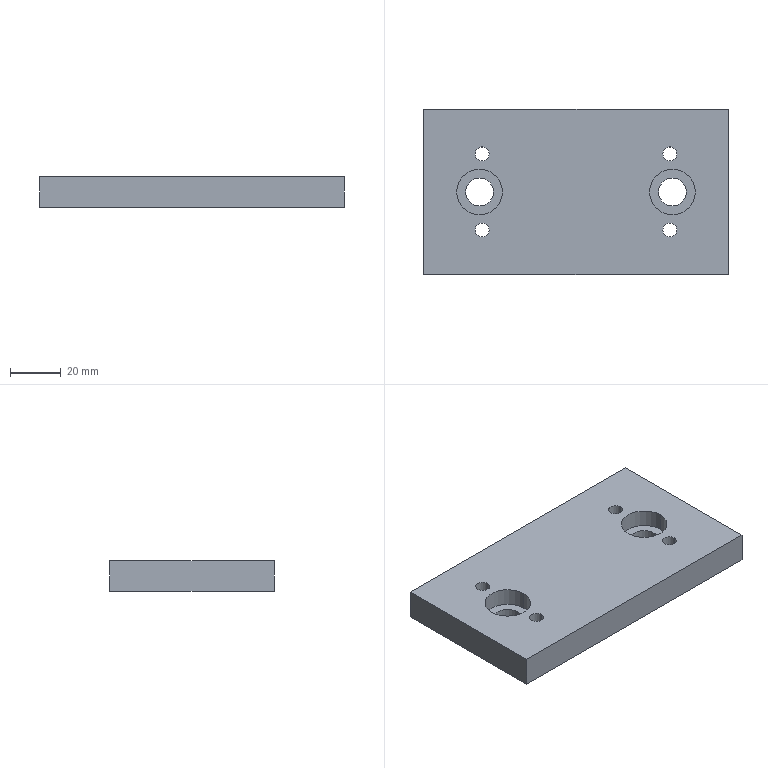Part | SolidWorks | features HoleWzd 2, Extrusion 1 | 1 solid | 36 faces | box 120 x 65 x 12 mm | volume 86698 mm3 | cylinder 24 | plane 12 | commonest cylinder face diameters 5.5 x8 10 x8 11 x4 18 x4
STEP:
#1=CARTESIAN_POINT('',(42.,15.,5.7));
#2=VERTEX_POINT('',#1);
#3=CARTESIAN_POINT('',(32.,15.,5.7));
#4=VERTEX_POINT('',#3);
#5=CARTESIAN_POINT('',(37.,15.,5.7));
#6=DIRECTION('',(0.,0.,-1.));
#7=DIRECTION('',(-1.,0.,0.));
#8=AXIS2_PLACEMENT_3D('',#5,#6,#7);
#9=CIRCLE('',#8,5.);
#10=EDGE_CURVE('',#2,#4,#9,.T.);
#11=ORIENTED_EDGE('',*,*,#10,.F.);
#12=CARTESIAN_POINT('',(42.,15.,0.));
#13=VERTEX_POINT('',#12);
#14=CARTESIAN_POINT('',(42.,15.,0.));
#15=DIRECTION('',(0.,0.,-1.));
#16=VECTOR('',#15,1000.);
#17=LINE('',#14,#16);
#18=EDGE_CURVE('',#2,#13,#17,.T.);
#19=ORIENTED_EDGE('',*,*,#18,.T.);
#20=CARTESIAN_POINT('',(32.,15.,0.));
#21=VERTEX_POINT('',#20);
#22=CARTESIAN_POINT('',(37.,15.,0.));
#23=DIRECTION('',(0.,0.,-1.));
#24=DIRECTION('',(-1.,0.,0.));
#25=AXIS2_PLACEMENT_3D('',#22,#23,#24);
#26=CIRCLE('',#25,5.);
#27=EDGE_CURVE('',#13,#21,#26,.T.);
#28=ORIENTED_EDGE('',*,*,#27,.T.);
#29=CARTESIAN_POINT('',(32.,15.,0.));
#30=DIRECTION('',(0.,0.,-1.));
#31=VECTOR('',#30,1000.);
#32=LINE('',#29,#31);
#33=EDGE_CURVE('',#4,#21,#32,.T.);
#34=ORIENTED_EDGE('',*,*,#33,.F.);
#35=EDGE_LOOP('',(#11,#19,#28,#34));
#36=FACE_OUTER_BOUND('',#35,.T.);
#37=CARTESIAN_POINT('',(37.,15.,0.));
#38=DIRECTION('',(0.,0.,-1.));
#39=DIRECTION('',(-1.,0.,0.));
#40=AXIS2_PLACEMENT_3D('',#37,#38,#39);
#41=CYLINDRICAL_SURFACE('',#40,5.);
#42=ADVANCED_FACE('',(#36),#41,.F.);
#43=CARTESIAN_POINT('',(39.75,15.,12.));
#44=VERTEX_POINT('',#43);
#45=CARTESIAN_POINT('',(34.25,15.,12.));
#46=VERTEX_POINT('',#45);
#47=CARTESIAN_POINT('',(37.,15.,12.));
#48=DIRECTION('',(0.,0.,-1.));
#49=DIRECTION('',(-1.,0.,0.));
#50=AXIS2_PLACEMENT_3D('',#47,#48,#49);
#51=CIRCLE('',#50,2.75);
#52=EDGE_CURVE('',#44,#46,#51,.T.);
#53=ORIENTED_EDGE('',*,*,#52,.F.);
#54=CARTESIAN_POINT('',(39.75,15.,5.7));
#55=VERTEX_POINT('',#54);
#56=CARTESIAN_POINT('',(39.75,15.,0.));
#57=DIRECTION('',(0.,0.,-1.));
#58=VECTOR('',#57,1000.);
#59=LINE('',#56,#58);
#60=EDGE_CURVE('',#44,#55,#59,.T.);
#61=ORIENTED_EDGE('',*,*,#60,.T.);
#62=CARTESIAN_POINT('',(34.25,15.,5.7));
#63=VERTEX_POINT('',#62);
#64=CARTESIAN_POINT('',(37.,15.,5.7));
#65=DIRECTION('',(0.,0.,-1.));
#66=DIRECTION('',(-1.,0.,0.));
#67=AXIS2_PLACEMENT_3D('',#64,#65,#66);
#68=CIRCLE('',#67,2.75);
#69=EDGE_CURVE('',#55,#63,#68,.T.);
#70=ORIENTED_EDGE('',*,*,#69,.T.);
#71=CARTESIAN_POINT('',(34.25,15.,0.));
#72=DIRECTION('',(0.,0.,-1.));
#73=VECTOR('',#72,1000.);
#74=LINE('',#71,#73);
#75=EDGE_CURVE('',#46,#63,#74,.T.);
#76=ORIENTED_EDGE('',*,*,#75,.F.);
#77=EDGE_LOOP('',(#53,#61,#70,#76));
#78=FACE_OUTER_BOUND('',#77,.T.);
#79=CARTESIAN_POINT('',(37.,15.,0.));
#80=DIRECTION('',(0.,0.,-1.));
#81=DIRECTION('',(-1.,0.,0.));
#82=AXIS2_PLACEMENT_3D('',#79,#80,#81);
#83=CYLINDRICAL_SURFACE('',#82,2.75);
#84=ADVANCED_FACE('',(#78),#83,.F.);
#85=CARTESIAN_POINT('',(42.,-15.,5.7));
#86=VERTEX_POINT('',#85);
#87=CARTESIAN_POINT('',(32.,-15.,5.7));
#88=VERTEX_POINT('',#87);
#89=CARTESIAN_POINT('',(37.,-15.,5.7));
#90=DIRECTION('',(0.,0.,-1.));
#91=DIRECTION('',(-1.,0.,0.));
#92=AXIS2_PLACEMENT_3D('',#89,#90,#91);
#93=CIRCLE('',#92,5.);
#94=EDGE_CURVE('',#86,#88,#93,.T.);
#95=ORIENTED_EDGE('',*,*,#94,.F.);
#96=CARTESIAN_POINT('',(42.,-15.,0.));
#97=VERTEX_POINT('',#96);
#98=CARTESIAN_POINT('',(42.,-15.,0.));
#99=DIRECTION('',(0.,0.,-1.));
#100=VECTOR('',#99,1000.);
#101=LINE('',#98,#100);
#102=EDGE_CURVE('',#86,#97,#101,.T.);
#103=ORIENTED_EDGE('',*,*,#102,.T.);
#104=CARTESIAN_POINT('',(32.,-15.,0.));
#105=VERTEX_POINT('',#104);
#106=CARTESIAN_POINT('',(37.,-15.,0.));
#107=DIRECTION('',(0.,0.,-1.));
#108=DIRECTION('',(-1.,0.,0.));
#109=AXIS2_PLACEMENT_3D('',#106,#107,#108);
#110=CIRCLE('',#109,5.);
#111=EDGE_CURVE('',#97,#105,#110,.T.);
#112=ORIENTED_EDGE('',*,*,#111,.T.);
#113=CARTESIAN_POINT('',(32.,-15.,0.));
#114=DIRECTION('',(0.,0.,-1.));
#115=VECTOR('',#114,1000.);
#116=LINE('',#113,#115);
#117=EDGE_CURVE('',#88,#105,#116,.T.);
#118=ORIENTED_EDGE('',*,*,#117,.F.);
#119=EDGE_LOOP('',(#95,#103,#112,#118));
#120=FACE_OUTER_BOUND('',#119,.T.);
#121=CARTESIAN_POINT('',(37.,-15.,0.));
#122=DIRECTION('',(0.,0.,-1.));
#123=DIRECTION('',(-1.,0.,0.));
#124=AXIS2_PLACEMENT_3D('',#121,#122,#123);
#125=CYLINDRICAL_SURFACE('',#124,5.);
#126=ADVANCED_FACE('',(#120),#125,.F.);
#127=CARTESIAN_POINT('',(39.75,-15.,12.));
#128=VERTEX_POINT('',#127);
#129=CARTESIAN_POINT('',(34.25,-15.,12.));
#130=VERTEX_POINT('',#129);
#131=CARTESIAN_POINT('',(37.,-15.,12.));
#132=DIRECTION('',(0.,0.,-1.));
#133=DIRECTION('',(-1.,0.,0.));
#134=AXIS2_PLACEMENT_3D('',#131,#132,#133);
#135=CIRCLE('',#134,2.75);
#136=EDGE_CURVE('',#128,#130,#135,.T.);
#137=ORIENTED_EDGE('',*,*,#136,.F.);
#138=CARTESIAN_POINT('',(39.75,-15.,5.7));
#139=VERTEX_POINT('',#138);
#140=CARTESIAN_POINT('',(39.75,-15.,0.));
#141=DIRECTION('',(0.,0.,-1.));
#142=VECTOR('',#141,1000.);
#143=LINE('',#140,#142);
#144=EDGE_CURVE('',#128,#139,#143,.T.);
#145=ORIENTED_EDGE('',*,*,#144,.T.);
#146=CARTESIAN_POINT('',(34.25,-15.,5.7));
#147=VERTEX_POINT('',#146);
#148=CARTESIAN_POINT('',(37.,-15.,5.7));
#149=DIRECTION('',(0.,0.,-1.));
#150=DIRECTION('',(-1.,0.,0.));
#151=AXIS2_PLACEMENT_3D('',#148,#149,#150);
#152=CIRCLE('',#151,2.75);
#153=EDGE_CURVE('',#139,#147,#152,.T.);
#154=ORIENTED_EDGE('',*,*,#153,.T.);
#155=CARTESIAN_POINT('',(34.25,-15.,0.));
#156=DIRECTION('',(0.,0.,-1.));
#157=VECTOR('',#156,1000.);
#158=LINE('',#155,#157);
#159=EDGE_CURVE('',#130,#147,#158,.T.);
#160=ORIENTED_EDGE('',*,*,#159,.F.);
#161=EDGE_LOOP('',(#137,#145,#154,#160));
#162=FACE_OUTER_BOUND('',#161,.T.);
#163=CARTESIAN_POINT('',(37.,-15.,0.));
#164=DIRECTION('',(0.,0.,-1.));
#165=DIRECTION('',(-1.,0.,0.));
#166=AXIS2_PLACEMENT_3D('',#163,#164,#165);
#167=CYLINDRICAL_SURFACE('',#166,2.75);
#168=ADVANCED_FACE('',(#162),#167,.F.);
#169=CARTESIAN_POINT('',(-32.,-15.,5.7));
#170=VERTEX_POINT('',#169);
#171=CARTESIAN_POINT('',(-42.,-15.,5.7));
#172=VERTEX_POINT('',#171);
#173=CARTESIAN_POINT('',(-37.,-15.,5.7));
#174=DIRECTION('',(0.,0.,-1.));
#175=DIRECTION('',(-1.,0.,0.));
#176=AXIS2_PLACEMENT_3D('',#173,#174,#175);
#177=CIRCLE('',#176,5.);
#178=EDGE_CURVE('',#170,#172,#177,.T.);
#179=ORIENTED_EDGE('',*,*,#178,.F.);
#180=CARTESIAN_POINT('',(-32.,-15.,0.));
#181=VERTEX_POINT('',#180);
#182=CARTESIAN_POINT('',(-32.,-15.,0.));
#183=DIRECTION('',(0.,0.,-1.));
#184=VECTOR('',#183,1000.);
#185=LINE('',#182,#184);
#186=EDGE_CURVE('',#170,#181,#185,.T.);
#187=ORIENTED_EDGE('',*,*,#186,.T.);
#188=CARTESIAN_POINT('',(-42.,-15.,0.));
#189=VERTEX_POINT('',#188);
#190=CARTESIAN_POINT('',(-37.,-15.,0.));
#191=DIRECTION('',(0.,0.,-1.));
#192=DIRECTION('',(-1.,0.,0.));
#193=AXIS2_PLACEMENT_3D('',#190,#191,#192);
#194=CIRCLE('',#193,5.);
#195=EDGE_CURVE('',#181,#189,#194,.T.);
#196=ORIENTED_EDGE('',*,*,#195,.T.);
#197=CARTESIAN_POINT('',(-42.,-15.,0.));
#198=DIRECTION('',(0.,0.,-1.));
#199=VECTOR('',#198,1000.);
#200=LINE('',#197,#199);
#201=EDGE_CURVE('',#172,#189,#200,.T.);
#202=ORIENTED_EDGE('',*,*,#201,.F.);
#203=EDGE_LOOP('',(#179,#187,#196,#202));
#204=FACE_OUTER_BOUND('',#203,.T.);
#205=CARTESIAN_POINT('',(-37.,-15.,0.));
#206=DIRECTION('',(0.,0.,-1.));
#207=DIRECTION('',(-1.,0.,0.));
#208=AXIS2_PLACEMENT_3D('',#205,#206,#207);
#209=CYLINDRICAL_SURFACE('',#208,5.);
#210=ADVANCED_FACE('',(#204),#209,.F.);
#211=CARTESIAN_POINT('',(-34.25,-15.,12.));
#212=VERTEX_POINT('',#211);
#213=CARTESIAN_POINT('',(-39.75,-15.,12.));
#214=VERTEX_POINT('',#213);
#215=CARTESIAN_POINT('',(-37.,-15.,12.));
#216=DIRECTION('',(0.,0.,-1.));
#217=DIRECTION('',(-1.,0.,0.));
#218=AXIS2_PLACEMENT_3D('',#215,#216,#217);
#219=CIRCLE('',#218,2.75);
#220=EDGE_CURVE('',#212,#214,#219,.T.);
#221=ORIENTED_EDGE('',*,*,#220,.F.);
#222=CARTESIAN_POINT('',(-34.25,-15.,5.7));
#223=VERTEX_POINT('',#222);
#224=CARTESIAN_POINT('',(-34.25,-15.,0.));
#225=DIRECTION('',(0.,0.,-1.));
#226=VECTOR('',#225,1000.);
#227=LINE('',#224,#226);
#228=EDGE_CURVE('',#212,#223,#227,.T.);
#229=ORIENTED_EDGE('',*,*,#228,.T.);
#230=CARTESIAN_POINT('',(-39.75,-15.,5.7));
#231=VERTEX_POINT('',#230);
#232=CARTESIAN_POINT('',(-37.,-15.,5.7));
#233=DIRECTION('',(0.,0.,-1.));
#234=DIRECTION('',(-1.,0.,0.));
#235=AXIS2_PLACEMENT_3D('',#232,#233,#234);
#236=CIRCLE('',#235,2.75);
#237=EDGE_CURVE('',#223,#231,#236,.T.);
#238=ORIENTED_EDGE('',*,*,#237,.T.);
#239=CARTESIAN_POINT('',(-39.75,-15.,0.));
#240=DIRECTION('',(0.,0.,-1.));
#241=VECTOR('',#240,1000.);
#242=LINE('',#239,#241);
#243=EDGE_CURVE('',#214,#231,#242,.T.);
#244=ORIENTED_EDGE('',*,*,#243,.F.);
#245=EDGE_LOOP('',(#221,#229,#238,#244));
#246=FACE_OUTER_BOUND('',#245,.T.);
#247=CARTESIAN_POINT('',(-37.,-15.,0.));
#248=DIRECTION('',(0.,0.,-1.));
#249=DIRECTION('',(-1.,0.,0.));
#250=AXIS2_PLACEMENT_3D('',#247,#248,#249);
#251=CYLINDRICAL_SURFACE('',#250,2.75);
#252=ADVANCED_FACE('',(#246),#251,.F.);
#253=CARTESIAN_POINT('',(-32.,15.,5.7));
#254=VERTEX_POINT('',#253);
#255=CARTESIAN_POINT('',(-42.,15.,5.7));
#256=VERTEX_POINT('',#255);
#257=CARTESIAN_POINT('',(-37.,15.,5.7));
#258=DIRECTION('',(0.,0.,-1.));
#259=DIRECTION('',(-1.,0.,0.));
#260=AXIS2_PLACEMENT_3D('',#257,#258,#259);
#261=CIRCLE('',#260,5.);
#262=EDGE_CURVE('',#254,#256,#261,.T.);
#263=ORIENTED_EDGE('',*,*,#262,.F.);
#264=CARTESIAN_POINT('',(-32.,15.,0.));
#265=VERTEX_POINT('',#264);
#266=CARTESIAN_POINT('',(-32.,15.,0.));
#267=DIRECTION('',(0.,0.,-1.));
#268=VECTOR('',#267,1000.);
#269=LINE('',#266,#268);
#270=EDGE_CURVE('',#254,#265,#269,.T.);
#271=ORIENTED_EDGE('',*,*,#270,.T.);
#272=CARTESIAN_POINT('',(-42.,15.,0.));
#273=VERTEX_POINT('',#272);
#274=CARTESIAN_POINT('',(-37.,15.,0.));
#275=DIRECTION('',(0.,0.,-1.));
#276=DIRECTION('',(-1.,0.,0.));
#277=AXIS2_PLACEMENT_3D('',#274,#275,#276);
#278=CIRCLE('',#277,5.);
#279=EDGE_CURVE('',#265,#273,#278,.T.);
#280=ORIENTED_EDGE('',*,*,#279,.T.);
#281=CARTESIAN_POINT('',(-42.,15.,0.));
#282=DIRECTION('',(0.,0.,-1.));
#283=VECTOR('',#282,1000.);
#284=LINE('',#281,#283);
#285=EDGE_CURVE('',#256,#273,#284,.T.);
#286=ORIENTED_EDGE('',*,*,#285,.F.);
#287=EDGE_LOOP('',(#263,#271,#280,#286));
#288=FACE_OUTER_BOUND('',#287,.T.);
#289=CARTESIAN_POINT('',(-37.,15.,0.));
#290=DIRECTION('',(0.,0.,-1.));
#291=DIRECTION('',(-1.,0.,0.));
#292=AXIS2_PLACEMENT_3D('',#289,#290,#291);
#293=CYLINDRICAL_SURFACE('',#292,5.);
#294=ADVANCED_FACE('',(#288),#293,.F.);
#295=CARTESIAN_POINT('',(-34.25,15.,12.));
#296=VERTEX_POINT('',#295);
#297=CARTESIAN_POINT('',(-39.75,15.,12.));
#298=VERTEX_POINT('',#297);
#299=CARTESIAN_POINT('',(-37.,15.,12.));
#300=DIRECTION('',(0.,0.,-1.));
#301=DIRECTION('',(-1.,0.,0.));
#302=AXIS2_PLACEMENT_3D('',#299,#300,#301);
#303=CIRCLE('',#302,2.75);
#304=EDGE_CURVE('',#296,#298,#303,.T.);
#305=ORIENTED_EDGE('',*,*,#304,.F.);
#306=CARTESIAN_POINT('',(-34.25,15.,5.7));
#307=VERTEX_POINT('',#306);
#308=CARTESIAN_POINT('',(-34.25,15.,0.));
#309=DIRECTION('',(0.,0.,-1.));
#310=VECTOR('',#309,1000.);
#311=LINE('',#308,#310);
#312=EDGE_CURVE('',#296,#307,#311,.T.);
#313=ORIENTED_EDGE('',*,*,#312,.T.);
#314=CARTESIAN_POINT('',(-39.75,15.,5.7));
#315=VERTEX_POINT('',#314);
#316=CARTESIAN_POINT('',(-37.,15.,5.7));
#317=DIRECTION('',(0.,0.,-1.));
#318=DIRECTION('',(-1.,0.,0.));
#319=AXIS2_PLACEMENT_3D('',#316,#317,#318);
#320=CIRCLE('',#319,2.75);
#321=EDGE_CURVE('',#307,#315,#320,.T.);
#322=ORIENTED_EDGE('',*,*,#321,.T.);
#323=CARTESIAN_POINT('',(-39.75,15.,0.));
#324=DIRECTION('',(0.,0.,-1.));
#325=VECTOR('',#324,1000.);
#326=LINE('',#323,#325);
#327=EDGE_CURVE('',#298,#315,#326,.T.);
#328=ORIENTED_EDGE('',*,*,#327,.F.);
#329=EDGE_LOOP('',(#305,#313,#322,#328));
#330=FACE_OUTER_BOUND('',#329,.T.);
#331=CARTESIAN_POINT('',(-37.,15.,0.));
#332=DIRECTION('',(0.,0.,-1.));
#333=DIRECTION('',(-1.,0.,0.));
#334=AXIS2_PLACEMENT_3D('',#331,#332,#333);
#335=CYLINDRICAL_SURFACE('',#334,2.75);
#336=ADVANCED_FACE('',(#330),#335,.F.);
#337=CARTESIAN_POINT('',(-47.,0.,5.));
#338=VERTEX_POINT('',#337);
#339=CARTESIAN_POINT('',(-29.,0.,5.));
#340=VERTEX_POINT('',#339);
#341=CARTESIAN_POINT('',(-38.,0.,5.));
#342=DIRECTION('',(0.,0.,1.));
#343=DIRECTION('',(1.,0.,0.));
#344=AXIS2_PLACEMENT_3D('',#341,#342,#343);
#345=CIRCLE('',#344,9.);
#346=EDGE_CURVE('',#338,#340,#345,.T.);
#347=ORIENTED_EDGE('',*,*,#346,.F.);
#348=CARTESIAN_POINT('',(-47.,0.,12.));
#349=VERTEX_POINT('',#348);
#350=CARTESIAN_POINT('',(-47.,0.,12.));
#351=DIRECTION('',(0.,0.,1.));
#352=VECTOR('',#351,1000.);
#353=LINE('',#350,#352);
#354=EDGE_CURVE('',#338,#349,#353,.T.);
#355=ORIENTED_EDGE('',*,*,#354,.T.);
#356=CARTESIAN_POINT('',(-29.,0.,12.));
#357=VERTEX_POINT('',#356);
#358=CARTESIAN_POINT('',(-38.,0.,12.));
#359=DIRECTION('',(0.,0.,1.));
#360=DIRECTION('',(1.,0.,0.));
#361=AXIS2_PLACEMENT_3D('',#358,#359,#360);
#362=CIRCLE('',#361,9.);
#363=EDGE_CURVE('',#349,#357,#362,.T.);
#364=ORIENTED_EDGE('',*,*,#363,.T.);
#365=CARTESIAN_POINT('',(-29.,0.,12.));
#366=DIRECTION('',(0.,0.,1.));
#367=VECTOR('',#366,1000.);
#368=LINE('',#365,#367);
#369=EDGE_CURVE('',#340,#357,#368,.T.);
#370=ORIENTED_EDGE('',*,*,#369,.F.);
#371=EDGE_LOOP('',(#347,#355,#364,#370));
#372=FACE_OUTER_BOUND('',#371,.T.);
#373=CARTESIAN_POINT('',(-38.,0.,12.));
#374=DIRECTION('',(0.,0.,1.));
#375=DIRECTION('',(1.,0.,0.));
#376=AXIS2_PLACEMENT_3D('',#373,#374,#375);
#377=CYLINDRICAL_SURFACE('',#376,9.);
#378=ADVANCED_FACE('',(#372),#377,.F.);
#379=CARTESIAN_POINT('',(-43.5,0.,0.));
#380=VERTEX_POINT('',#379);
#381=CARTESIAN_POINT('',(-32.5,0.,0.));
#382=VERTEX_POINT('',#381);
#383=CARTESIAN_POINT('',(-38.,0.,0.));
#384=DIRECTION('',(0.,0.,1.));
#385=DIRECTION('',(1.,0.,0.));
#386=AXIS2_PLACEMENT_3D('',#383,#384,#385);
#387=CIRCLE('',#386,5.5);
#388=EDGE_CURVE('',#380,#382,#387,.T.);
#389=ORIENTED_EDGE('',*,*,#388,.F.);
#390=CARTESIAN_POINT('',(-43.5,0.,5.));
#391=VERTEX_POINT('',#390);
#392=CARTESIAN_POINT('',(-43.5,0.,12.));
#393=DIRECTION('',(0.,0.,1.));
#394=VECTOR('',#393,1000.);
#395=LINE('',#392,#394);
#396=EDGE_CURVE('',#380,#391,#395,.T.);
#397=ORIENTED_EDGE('',*,*,#396,.T.);
#398=CARTESIAN_POINT('',(-32.5,0.,5.));
#399=VERTEX_POINT('',#398);
#400=CARTESIAN_POINT('',(-38.,0.,5.));
#401=DIRECTION('',(0.,0.,1.));
#402=DIRECTION('',(1.,0.,0.));
#403=AXIS2_PLACEMENT_3D('',#400,#401,#402);
#404=CIRCLE('',#403,5.5);
#405=EDGE_CURVE('',#391,#399,#404,.T.);
#406=ORIENTED_EDGE('',*,*,#405,.T.);
#407=CARTESIAN_POINT('',(-32.5,0.,12.));
#408=DIRECTION('',(0.,0.,1.));
#409=VECTOR('',#408,1000.);
#410=LINE('',#407,#409);
#411=EDGE_CURVE('',#382,#399,#410,.T.);
#412=ORIENTED_EDGE('',*,*,#411,.F.);
#413=EDGE_LOOP('',(#389,#397,#406,#412));
#414=FACE_OUTER_BOUND('',#413,.T.);
#415=CARTESIAN_POINT('',(-38.,0.,12.));
#416=DIRECTION('',(0.,0.,1.));
#417=DIRECTION('',(1.,0.,0.));
#418=AXIS2_PLACEMENT_3D('',#415,#416,#417);
#419=CYLINDRICAL_SURFACE('',#418,5.5);
#420=ADVANCED_FACE('',(#414),#419,.F.);
#421=CARTESIAN_POINT('',(29.,0.,5.));
#422=VERTEX_POINT('',#421);
#423=CARTESIAN_POINT('',(47.,0.,5.));
#424=VERTEX_POINT('',#423);
#425=CARTESIAN_POINT('',(38.,0.,5.));
#426=DIRECTION('',(0.,0.,1.));
#427=DIRECTION('',(1.,0.,0.));
#428=AXIS2_PLACEMENT_3D('',#425,#426,#427);
#429=CIRCLE('',#428,9.);
#430=EDGE_CURVE('',#422,#424,#429,.T.);
#431=ORIENTED_EDGE('',*,*,#430,.F.);
#432=CARTESIAN_POINT('',(29.,0.,12.));
#433=VERTEX_POINT('',#432);
#434=CARTESIAN_POINT('',(29.,0.,12.));
#435=DIRECTION('',(0.,0.,1.));
#436=VECTOR('',#435,1000.);
#437=LINE('',#434,#436);
#438=EDGE_CURVE('',#422,#433,#437,.T.);
#439=ORIENTED_EDGE('',*,*,#438,.T.);
#440=CARTESIAN_POINT('',(47.,0.,12.));
#441=VERTEX_POINT('',#440);
#442=CARTESIAN_POINT('',(38.,0.,12.));
#443=DIRECTION('',(0.,0.,1.));
#444=DIRECTION('',(1.,0.,0.));
#445=AXIS2_PLACEMENT_3D('',#442,#443,#444);
#446=CIRCLE('',#445,9.);
#447=EDGE_CURVE('',#433,#441,#446,.T.);
#448=ORIENTED_EDGE('',*,*,#447,.T.);
#449=CARTESIAN_POINT('',(47.,0.,12.));
#450=DIRECTION('',(0.,0.,1.));
#451=VECTOR('',#450,1000.);
#452=LINE('',#449,#451);
#453=EDGE_CURVE('',#424,#441,#452,.T.);
#454=ORIENTED_EDGE('',*,*,#453,.F.);
#455=EDGE_LOOP('',(#431,#439,#448,#454));
#456=FACE_OUTER_BOUND('',#455,.T.);
#457=CARTESIAN_POINT('',(38.,0.,12.));
#458=DIRECTION('',(0.,0.,1.));
#459=DIRECTION('',(1.,0.,0.));
#460=AXIS2_PLACEMENT_3D('',#457,#458,#459);
#461=CYLINDRICAL_SURFACE('',#460,9.);
#462=ADVANCED_FACE('',(#456),#461,.F.);
#463=CARTESIAN_POINT('',(32.5,0.,0.));
#464=VERTEX_POINT('',#463);
#465=CARTESIAN_POINT('',(43.5,0.,0.));
#466=VERTEX_POINT('',#465);
#467=CARTESIAN_POINT('',(38.,0.,0.));
#468=DIRECTION('',(0.,0.,1.));
#469=DIRECTION('',(1.,0.,0.));
#470=AXIS2_PLACEMENT_3D('',#467,#468,#469);
#471=CIRCLE('',#470,5.5);
#472=EDGE_CURVE('',#464,#466,#471,.T.);
#473=ORIENTED_EDGE('',*,*,#472,.F.);
#474=CARTESIAN_POINT('',(32.5,0.,5.));
#475=VERTEX_POINT('',#474);
#476=CARTESIAN_POINT('',(32.5,0.,12.));
#477=DIRECTION('',(0.,0.,1.));
#478=VECTOR('',#477,1000.);
#479=LINE('',#476,#478);
#480=EDGE_CURVE('',#464,#475,#479,.T.);
#481=ORIENTED_EDGE('',*,*,#480,.T.);
#482=CARTESIAN_POINT('',(43.5,0.,5.));
#483=VERTEX_POINT('',#482);
#484=CARTESIAN_POINT('',(38.,0.,5.));
#485=DIRECTION('',(0.,0.,1.));
#486=DIRECTION('',(1.,0.,0.));
#487=AXIS2_PLACEMENT_3D('',#484,#485,#486);
#488=CIRCLE('',#487,5.5);
#489=EDGE_CURVE('',#475,#483,#488,.T.);
#490=ORIENTED_EDGE('',*,*,#489,.T.);
#491=CARTESIAN_POINT('',(43.5,0.,12.));
#492=DIRECTION('',(0.,0.,1.));
#493=VECTOR('',#492,1000.);
#494=LINE('',#491,#493);
#495=EDGE_CURVE('',#466,#483,#494,.T.);
#496=ORIENTED_EDGE('',*,*,#495,.F.);
#497=EDGE_LOOP('',(#473,#481,#490,#496));
#498=FACE_OUTER_BOUND('',#497,.T.);
#499=CARTESIAN_POINT('',(38.,0.,12.));
#500=DIRECTION('',(0.,0.,1.));
#501=DIRECTION('',(1.,0.,0.));
#502=AXIS2_PLACEMENT_3D('',#499,#500,#501);
#503=CYLINDRICAL_SURFACE('',#502,5.5);
#504=ADVANCED_FACE('',(#498),#503,.F.);
#505=CARTESIAN_POINT('',(60.,-32.5,0.));
#506=VERTEX_POINT('',#505);
#507=CARTESIAN_POINT('',(60.,32.5,0.));
#508=VERTEX_POINT('',#507);
#509=CARTESIAN_POINT('',(60.,32.5,0.));
#510=DIRECTION('',(0.,1.,0.));
#511=VECTOR('',#510,1000.);
#512=LINE('',#509,#511);
#513=EDGE_CURVE('',#506,#508,#512,.T.);
#514=ORIENTED_EDGE('',*,*,#513,.T.);
#515=CARTESIAN_POINT('',(60.,32.5,12.));
#516=VERTEX_POINT('',#515);
#517=CARTESIAN_POINT('',(60.,32.5,12.));
#518=DIRECTION('',(0.,0.,-1.));
#519=VECTOR('',#518,1000.);
#520=LINE('',#517,#519);
#521=EDGE_CURVE('',#516,#508,#520,.T.);
#522=ORIENTED_EDGE('',*,*,#521,.F.);
#523=CARTESIAN_POINT('',(60.,-32.5,12.));
#524=VERTEX_POINT('',#523);
#525=CARTESIAN_POINT('',(60.,32.5,12.));
#526=DIRECTION('',(0.,1.,0.));
#527=VECTOR('',#526,1000.);
#528=LINE('',#525,#527);
#529=EDGE_CURVE('',#524,#516,#528,.T.);
#530=ORIENTED_EDGE('',*,*,#529,.F.);
#531=CARTESIAN_POINT('',(60.,-32.5,12.));
#532=DIRECTION('',(0.,0.,-1.));
#533=VECTOR('',#532,1000.);
#534=LINE('',#531,#533);
#535=EDGE_CURVE('',#524,#506,#534,.T.);
#536=ORIENTED_EDGE('',*,*,#535,.T.);
#537=EDGE_LOOP('',(#514,#522,#530,#536));
#538=FACE_OUTER_BOUND('',#537,.T.);
#539=CARTESIAN_POINT('',(60.,32.5,12.));
#540=DIRECTION('',(-1.,0.,0.));
#541=DIRECTION('',(0.,-1.,0.));
#542=AXIS2_PLACEMENT_3D('',#539,#540,#541);
#543=PLANE('',#542);
#544=ADVANCED_FACE('',(#538),#543,.F.);
#545=CARTESIAN_POINT('',(-60.,32.5,0.));
#546=VERTEX_POINT('',#545);
#547=CARTESIAN_POINT('',(-60.,32.5,0.));
#548=DIRECTION('',(-1.,0.,0.));
#549=VECTOR('',#548,1000.);
#550=LINE('',#547,#549);
#551=EDGE_CURVE('',#508,#546,#550,.T.);
#552=ORIENTED_EDGE('',*,*,#551,.T.);
#553=CARTESIAN_POINT('',(-60.,32.5,12.));
#554=VERTEX_POINT('',#553);
#555=CARTESIAN_POINT('',(-60.,32.5,12.));
#556=DIRECTION('',(0.,0.,-1.));
#557=VECTOR('',#556,1000.);
#558=LINE('',#555,#557);
#559=EDGE_CURVE('',#554,#546,#558,.T.);
#560=ORIENTED_EDGE('',*,*,#559,.F.);
#561=CARTESIAN_POINT('',(-60.,32.5,12.));
#562=DIRECTION('',(-1.,0.,0.));
#563=VECTOR('',#562,1000.);
#564=LINE('',#561,#563);
#565=EDGE_CURVE('',#516,#554,#564,.T.);
#566=ORIENTED_EDGE('',*,*,#565,.F.);
#567=ORIENTED_EDGE('',*,*,#521,.T.);
#568=EDGE_LOOP('',(#552,#560,#566,#567));
#569=FACE_OUTER_BOUND('',#568,.T.);
#570=CARTESIAN_POINT('',(-60.,32.5,12.));
#571=DIRECTION('',(0.,-1.,0.));
#572=DIRECTION('',(0.,0.,-1.));
#573=AXIS2_PLACEMENT_3D('',#570,#571,#572);
#574=PLANE('',#573);
#575=ADVANCED_FACE('',(#569),#574,.F.);
#576=CARTESIAN_POINT('',(-60.,-32.5,0.));
#577=VERTEX_POINT('',#576);
#578=CARTESIAN_POINT('',(-60.,32.5,0.));
#579=DIRECTION('',(0.,-1.,0.));
#580=VECTOR('',#579,1000.);
#581=LINE('',#578,#580);
#582=EDGE_CURVE('',#546,#577,#581,.T.);
#583=ORIENTED_EDGE('',*,*,#582,.T.);
#584=CARTESIAN_POINT('',(-60.,-32.5,12.));
#585=VERTEX_POINT('',#584);
#586=CARTESIAN_POINT('',(-60.,-32.5,12.));
#587=DIRECTION('',(0.,0.,-1.));
#588=VECTOR('',#587,1000.);
#589=LINE('',#586,#588);
#590=EDGE_CURVE('',#585,#577,#589,.T.);
#591=ORIENTED_EDGE('',*,*,#590,.F.);
#592=CARTESIAN_POINT('',(-60.,32.5,12.));
#593=DIRECTION('',(0.,-1.,0.));
#594=VECTOR('',#593,1000.);
#595=LINE('',#592,#594);
#596=EDGE_CURVE('',#554,#585,#595,.T.);
#597=ORIENTED_EDGE('',*,*,#596,.F.);
#598=ORIENTED_EDGE('',*,*,#559,.T.);
#599=EDGE_LOOP('',(#583,#591,#597,#598));
#600=FACE_OUTER_BOUND('',#599,.T.);
#601=CARTESIAN_POINT('',(-60.,32.5,12.));
#602=DIRECTION('',(1.,0.,0.));
#603=DIRECTION('',(0.,1.,0.));
#604=AXIS2_PLACEMENT_3D('',#601,#602,#603);
#605=PLANE('',#604);
#606=ADVANCED_FACE('',(#600),#605,.F.);
#607=CARTESIAN_POINT('',(-60.,-32.5,0.));
#608=DIRECTION('',(1.,0.,0.));
#609=VECTOR('',#608,1000.);
#610=LINE('',#607,#609);
#611=EDGE_CURVE('',#577,#506,#610,.T.);
#612=ORIENTED_EDGE('',*,*,#611,.T.);
#613=ORIENTED_EDGE('',*,*,#535,.F.);
#614=CARTESIAN_POINT('',(-60.,-32.5,12.));
#615=DIRECTION('',(1.,0.,0.));
#616=VECTOR('',#615,1000.);
#617=LINE('',#614,#616);
#618=EDGE_CURVE('',#585,#524,#617,.T.);
#619=ORIENTED_EDGE('',*,*,#618,.F.);
#620=ORIENTED_EDGE('',*,*,#590,.T.);
#621=EDGE_LOOP('',(#612,#613,#619,#620));
#622=FACE_OUTER_BOUND('',#621,.T.);
#623=CARTESIAN_POINT('',(-60.,-32.5,12.));
#624=DIRECTION('',(0.,1.,0.));
#625=DIRECTION('',(0.,0.,1.));
#626=AXIS2_PLACEMENT_3D('',#623,#624,#625);
#627=PLANE('',#626);
#628=ADVANCED_FACE('',(#622),#627,.F.);
#629=CARTESIAN_POINT('',(37.,15.,12.));
#630=DIRECTION('',(0.,0.,-1.));
#631=DIRECTION('',(-1.,0.,0.));
#632=AXIS2_PLACEMENT_3D('',#629,#630,#631);
#633=CIRCLE('',#632,2.75);
#634=EDGE_CURVE('',#46,#44,#633,.T.);
#635=ORIENTED_EDGE('',*,*,#634,.T.);
#636=ORIENTED_EDGE('',*,*,#52,.T.);
#637=EDGE_LOOP('',(#635,#636));
#638=FACE_BOUND('',#637,.T.);
#639=CARTESIAN_POINT('',(37.,-15.,12.));
#640=DIRECTION('',(0.,0.,-1.));
#641=DIRECTION('',(-1.,0.,0.));
#642=AXIS2_PLACEMENT_3D('',#639,#640,#641);
#643=CIRCLE('',#642,2.75);
#644=EDGE_CURVE('',#130,#128,#643,.T.);
#645=ORIENTED_EDGE('',*,*,#644,.T.);
#646=ORIENTED_EDGE('',*,*,#136,.T.);
#647=EDGE_LOOP('',(#645,#646));
#648=FACE_BOUND('',#647,.T.);
#649=CARTESIAN_POINT('',(-37.,-15.,12.));
#650=DIRECTION('',(0.,0.,-1.));
#651=DIRECTION('',(-1.,0.,0.));
#652=AXIS2_PLACEMENT_3D('',#649,#650,#651);
#653=CIRCLE('',#652,2.75);
#654=EDGE_CURVE('',#214,#212,#653,.T.);
#655=ORIENTED_EDGE('',*,*,#654,.T.);
#656=ORIENTED_EDGE('',*,*,#220,.T.);
#657=EDGE_LOOP('',(#655,#656));
#658=FACE_BOUND('',#657,.T.);
#659=CARTESIAN_POINT('',(-37.,15.,12.));
#660=DIRECTION('',(0.,0.,-1.));
#661=DIRECTION('',(-1.,0.,0.));
#662=AXIS2_PLACEMENT_3D('',#659,#660,#661);
#663=CIRCLE('',#662,2.75);
#664=EDGE_CURVE('',#298,#296,#663,.T.);
#665=ORIENTED_EDGE('',*,*,#664,.T.);
#666=ORIENTED_EDGE('',*,*,#304,.T.);
#667=EDGE_LOOP('',(#665,#666));
#668=FACE_BOUND('',#667,.T.);
#669=CARTESIAN_POINT('',(-38.,0.,12.));
#670=DIRECTION('',(0.,0.,1.));
#671=DIRECTION('',(1.,0.,0.));
#672=AXIS2_PLACEMENT_3D('',#669,#670,#671);
#673=CIRCLE('',#672,9.);
#674=EDGE_CURVE('',#357,#349,#673,.T.);
#675=ORIENTED_EDGE('',*,*,#674,.F.);
#676=ORIENTED_EDGE('',*,*,#363,.F.);
#677=EDGE_LOOP('',(#675,#676));
#678=FACE_BOUND('',#677,.T.);
#679=CARTESIAN_POINT('',(38.,0.,12.));
#680=DIRECTION('',(0.,0.,1.));
#681=DIRECTION('',(1.,0.,0.));
#682=AXIS2_PLACEMENT_3D('',#679,#680,#681);
#683=CIRCLE('',#682,9.);
#684=EDGE_CURVE('',#441,#433,#683,.T.);
#685=ORIENTED_EDGE('',*,*,#684,.F.);
#686=ORIENTED_EDGE('',*,*,#447,.F.);
#687=EDGE_LOOP('',(#685,#686));
#688=FACE_BOUND('',#687,.T.);
#689=ORIENTED_EDGE('',*,*,#529,.T.);
#690=ORIENTED_EDGE('',*,*,#565,.T.);
#691=ORIENTED_EDGE('',*,*,#596,.T.);
#692=ORIENTED_EDGE('',*,*,#618,.T.);
#693=EDGE_LOOP('',(#689,#690,#691,#692));
#694=FACE_OUTER_BOUND('',#693,.T.);
#695=CARTESIAN_POINT('',(0.,0.,12.));
#696=DIRECTION('',(0.,0.,1.));
#697=DIRECTION('',(1.,0.,0.));
#698=AXIS2_PLACEMENT_3D('',#695,#696,#697);
#699=PLANE('',#698);
#700=ADVANCED_FACE('',(#638,#648,#658,#668,#678,#688,#694),#699,.T.);
#701=CARTESIAN_POINT('',(37.,15.,0.));
#702=DIRECTION('',(0.,0.,-1.));
#703=DIRECTION('',(-1.,0.,0.));
#704=AXIS2_PLACEMENT_3D('',#701,#702,#703);
#705=CIRCLE('',#704,5.);
#706=EDGE_CURVE('',#21,#13,#705,.T.);
#707=ORIENTED_EDGE('',*,*,#706,.F.);
#708=ORIENTED_EDGE('',*,*,#27,.F.);
#709=EDGE_LOOP('',(#707,#708));
#710=FACE_BOUND('',#709,.T.);
#711=CARTESIAN_POINT('',(37.,-15.,0.));
#712=DIRECTION('',(0.,0.,-1.));
#713=DIRECTION('',(-1.,0.,0.));
#714=AXIS2_PLACEMENT_3D('',#711,#712,#713);
#715=CIRCLE('',#714,5.);
#716=EDGE_CURVE('',#105,#97,#715,.T.);
#717=ORIENTED_EDGE('',*,*,#716,.F.);
#718=ORIENTED_EDGE('',*,*,#111,.F.);
#719=EDGE_LOOP('',(#717,#718));
#720=FACE_BOUND('',#719,.T.);
#721=CARTESIAN_POINT('',(-37.,-15.,0.));
#722=DIRECTION('',(0.,0.,-1.));
#723=DIRECTION('',(-1.,0.,0.));
#724=AXIS2_PLACEMENT_3D('',#721,#722,#723);
#725=CIRCLE('',#724,5.);
#726=EDGE_CURVE('',#189,#181,#725,.T.);
#727=ORIENTED_EDGE('',*,*,#726,.F.);
#728=ORIENTED_EDGE('',*,*,#195,.F.);
#729=EDGE_LOOP('',(#727,#728));
#730=FACE_BOUND('',#729,.T.);
#731=CARTESIAN_POINT('',(-37.,15.,0.));
#732=DIRECTION('',(0.,0.,-1.));
#733=DIRECTION('',(-1.,0.,0.));
#734=AXIS2_PLACEMENT_3D('',#731,#732,#733);
#735=CIRCLE('',#734,5.);
#736=EDGE_CURVE('',#273,#265,#735,.T.);
#737=ORIENTED_EDGE('',*,*,#736,.F.);
#738=ORIENTED_EDGE('',*,*,#279,.F.);
#739=EDGE_LOOP('',(#737,#738));
#740=FACE_BOUND('',#739,.T.);
#741=CARTESIAN_POINT('',(-38.,0.,0.));
#742=DIRECTION('',(0.,0.,1.));
#743=DIRECTION('',(1.,0.,0.));
#744=AXIS2_PLACEMENT_3D('',#741,#742,#743);
#745=CIRCLE('',#744,5.5);
#746=EDGE_CURVE('',#382,#380,#745,.T.);
#747=ORIENTED_EDGE('',*,*,#746,.T.);
#748=ORIENTED_EDGE('',*,*,#388,.T.);
#749=EDGE_LOOP('',(#747,#748));
#750=FACE_BOUND('',#749,.T.);
#751=CARTESIAN_POINT('',(38.,0.,0.));
#752=DIRECTION('',(0.,0.,1.));
#753=DIRECTION('',(1.,0.,0.));
#754=AXIS2_PLACEMENT_3D('',#751,#752,#753);
#755=CIRCLE('',#754,5.5);
#756=EDGE_CURVE('',#466,#464,#755,.T.);
#757=ORIENTED_EDGE('',*,*,#756,.T.);
#758=ORIENTED_EDGE('',*,*,#472,.T.);
#759=EDGE_LOOP('',(#757,#758));
#760=FACE_BOUND('',#759,.T.);
#761=ORIENTED_EDGE('',*,*,#513,.F.);
#762=ORIENTED_EDGE('',*,*,#611,.F.);
#763=ORIENTED_EDGE('',*,*,#582,.F.);
#764=ORIENTED_EDGE('',*,*,#551,.F.);
#765=EDGE_LOOP('',(#761,#762,#763,#764));
#766=FACE_OUTER_BOUND('',#765,.T.);
#767=CARTESIAN_POINT('',(0.,0.,0.));
#768=DIRECTION('',(0.,0.,1.));
#769=DIRECTION('',(1.,0.,0.));
#770=AXIS2_PLACEMENT_3D('',#767,#768,#769);
#771=PLANE('',#770);
#772=ADVANCED_FACE('',(#710,#720,#730,#740,#750,#760,#766),#771,.F.);
#773=ORIENTED_EDGE('',*,*,#480,.F.);
#774=ORIENTED_EDGE('',*,*,#756,.F.);
#775=ORIENTED_EDGE('',*,*,#495,.T.);
#776=CARTESIAN_POINT('',(38.,0.,5.));
#777=DIRECTION('',(0.,0.,1.));
#778=DIRECTION('',(1.,0.,0.));
#779=AXIS2_PLACEMENT_3D('',#776,#777,#778);
#780=CIRCLE('',#779,5.5);
#781=EDGE_CURVE('',#483,#475,#780,.T.);
#782=ORIENTED_EDGE('',*,*,#781,.T.);
#783=EDGE_LOOP('',(#773,#774,#775,#782));
#784=FACE_OUTER_BOUND('',#783,.T.);
#785=CARTESIAN_POINT('',(38.,0.,12.));
#786=DIRECTION('',(0.,0.,1.));
#787=DIRECTION('',(1.,0.,0.));
#788=AXIS2_PLACEMENT_3D('',#785,#786,#787);
#789=CYLINDRICAL_SURFACE('',#788,5.5);
#790=ADVANCED_FACE('',(#784),#789,.F.);
#791=ORIENTED_EDGE('',*,*,#781,.F.);
#792=ORIENTED_EDGE('',*,*,#489,.F.);
#793=EDGE_LOOP('',(#791,#792));
#794=FACE_BOUND('',#793,.T.);
#795=CARTESIAN_POINT('',(38.,0.,5.));
#796=DIRECTION('',(0.,0.,1.));
#797=DIRECTION('',(1.,0.,0.));
#798=AXIS2_PLACEMENT_3D('',#795,#796,#797);
#799=CIRCLE('',#798,9.);
#800=EDGE_CURVE('',#424,#422,#799,.T.);
#801=ORIENTED_EDGE('',*,*,#800,.T.);
#802=ORIENTED_EDGE('',*,*,#430,.T.);
#803=EDGE_LOOP('',(#801,#802));
#804=FACE_OUTER_BOUND('',#803,.T.);
#805=CARTESIAN_POINT('',(43.5,0.,5.));
#806=DIRECTION('',(0.,0.,-1.));
#807=DIRECTION('',(-1.,0.,0.));
#808=AXIS2_PLACEMENT_3D('',#805,#806,#807);
#809=PLANE('',#808);
#810=ADVANCED_FACE('',(#794,#804),#809,.F.);
#811=ORIENTED_EDGE('',*,*,#438,.F.);
#812=ORIENTED_EDGE('',*,*,#800,.F.);
#813=ORIENTED_EDGE('',*,*,#453,.T.);
#814=ORIENTED_EDGE('',*,*,#684,.T.);
#815=EDGE_LOOP('',(#811,#812,#813,#814));
#816=FACE_OUTER_BOUND('',#815,.T.);
#817=CARTESIAN_POINT('',(38.,0.,12.));
#818=DIRECTION('',(0.,0.,1.));
#819=DIRECTION('',(1.,0.,0.));
#820=AXIS2_PLACEMENT_3D('',#817,#818,#819);
#821=CYLINDRICAL_SURFACE('',#820,9.);
#822=ADVANCED_FACE('',(#816),#821,.F.);
#823=ORIENTED_EDGE('',*,*,#396,.F.);
#824=ORIENTED_EDGE('',*,*,#746,.F.);
#825=ORIENTED_EDGE('',*,*,#411,.T.);
#826=CARTESIAN_POINT('',(-38.,0.,5.));
#827=DIRECTION('',(0.,0.,1.));
#828=DIRECTION('',(1.,0.,0.));
#829=AXIS2_PLACEMENT_3D('',#826,#827,#828);
#830=CIRCLE('',#829,5.5);
#831=EDGE_CURVE('',#399,#391,#830,.T.);
#832=ORIENTED_EDGE('',*,*,#831,.T.);
#833=EDGE_LOOP('',(#823,#824,#825,#832));
#834=FACE_OUTER_BOUND('',#833,.T.);
#835=CARTESIAN_POINT('',(-38.,0.,12.));
#836=DIRECTION('',(0.,0.,1.));
#837=DIRECTION('',(1.,0.,0.));
#838=AXIS2_PLACEMENT_3D('',#835,#836,#837);
#839=CYLINDRICAL_SURFACE('',#838,5.5);
#840=ADVANCED_FACE('',(#834),#839,.F.);
#841=ORIENTED_EDGE('',*,*,#831,.F.);
#842=ORIENTED_EDGE('',*,*,#405,.F.);
#843=EDGE_LOOP('',(#841,#842));
#844=FACE_BOUND('',#843,.T.);
#845=CARTESIAN_POINT('',(-38.,0.,5.));
#846=DIRECTION('',(0.,0.,1.));
#847=DIRECTION('',(1.,0.,0.));
#848=AXIS2_PLACEMENT_3D('',#845,#846,#847);
#849=CIRCLE('',#848,9.);
#850=EDGE_CURVE('',#340,#338,#849,.T.);
#851=ORIENTED_EDGE('',*,*,#850,.T.);
#852=ORIENTED_EDGE('',*,*,#346,.T.);
#853=EDGE_LOOP('',(#851,#852));
#854=FACE_OUTER_BOUND('',#853,.T.);
#855=CARTESIAN_POINT('',(-32.5,0.,5.));
#856=DIRECTION('',(0.,0.,-1.));
#857=DIRECTION('',(-1.,0.,0.));
#858=AXIS2_PLACEMENT_3D('',#855,#856,#857);
#859=PLANE('',#858);
#860=ADVANCED_FACE('',(#844,#854),#859,.F.);
#861=ORIENTED_EDGE('',*,*,#354,.F.);
#862=ORIENTED_EDGE('',*,*,#850,.F.);
#863=ORIENTED_EDGE('',*,*,#369,.T.);
#864=ORIENTED_EDGE('',*,*,#674,.T.);
#865=EDGE_LOOP('',(#861,#862,#863,#864));
#866=FACE_OUTER_BOUND('',#865,.T.);
#867=CARTESIAN_POINT('',(-38.,0.,12.));
#868=DIRECTION('',(0.,0.,1.));
#869=DIRECTION('',(1.,0.,0.));
#870=AXIS2_PLACEMENT_3D('',#867,#868,#869);
#871=CYLINDRICAL_SURFACE('',#870,9.);
#872=ADVANCED_FACE('',(#866),#871,.F.);
#873=ORIENTED_EDGE('',*,*,#312,.F.);
#874=ORIENTED_EDGE('',*,*,#664,.F.);
#875=ORIENTED_EDGE('',*,*,#327,.T.);
#876=CARTESIAN_POINT('',(-37.,15.,5.7));
#877=DIRECTION('',(0.,0.,-1.));
#878=DIRECTION('',(-1.,0.,0.));
#879=AXIS2_PLACEMENT_3D('',#876,#877,#878);
#880=CIRCLE('',#879,2.75);
#881=EDGE_CURVE('',#315,#307,#880,.T.);
#882=ORIENTED_EDGE('',*,*,#881,.T.);
#883=EDGE_LOOP('',(#873,#874,#875,#882));
#884=FACE_OUTER_BOUND('',#883,.T.);
#885=CARTESIAN_POINT('',(-37.,15.,0.));
#886=DIRECTION('',(0.,0.,-1.));
#887=DIRECTION('',(-1.,0.,0.));
#888=AXIS2_PLACEMENT_3D('',#885,#886,#887);
#889=CYLINDRICAL_SURFACE('',#888,2.75);
#890=ADVANCED_FACE('',(#884),#889,.F.);
#891=ORIENTED_EDGE('',*,*,#881,.F.);
#892=ORIENTED_EDGE('',*,*,#321,.F.);
#893=EDGE_LOOP('',(#891,#892));
#894=FACE_BOUND('',#893,.T.);
#895=CARTESIAN_POINT('',(-37.,15.,5.7));
#896=DIRECTION('',(0.,0.,-1.));
#897=DIRECTION('',(-1.,0.,0.));
#898=AXIS2_PLACEMENT_3D('',#895,#896,#897);
#899=CIRCLE('',#898,5.);
#900=EDGE_CURVE('',#256,#254,#899,.T.);
#901=ORIENTED_EDGE('',*,*,#900,.T.);
#902=ORIENTED_EDGE('',*,*,#262,.T.);
#903=EDGE_LOOP('',(#901,#902));
#904=FACE_OUTER_BOUND('',#903,.T.);
#905=CARTESIAN_POINT('',(-34.25,15.,5.7));
#906=DIRECTION('',(0.,0.,1.));
#907=DIRECTION('',(1.,0.,0.));
#908=AXIS2_PLACEMENT_3D('',#905,#906,#907);
#909=PLANE('',#908);
#910=ADVANCED_FACE('',(#894,#904),#909,.F.);
#911=ORIENTED_EDGE('',*,*,#270,.F.);
#912=ORIENTED_EDGE('',*,*,#900,.F.);
#913=ORIENTED_EDGE('',*,*,#285,.T.);
#914=ORIENTED_EDGE('',*,*,#736,.T.);
#915=EDGE_LOOP('',(#911,#912,#913,#914));
#916=FACE_OUTER_BOUND('',#915,.T.);
#917=CARTESIAN_POINT('',(-37.,15.,0.));
#918=DIRECTION('',(0.,0.,-1.));
#919=DIRECTION('',(-1.,0.,0.));
#920=AXIS2_PLACEMENT_3D('',#917,#918,#919);
#921=CYLINDRICAL_SURFACE('',#920,5.);
#922=ADVANCED_FACE('',(#916),#921,.F.);
#923=ORIENTED_EDGE('',*,*,#228,.F.);
#924=ORIENTED_EDGE('',*,*,#654,.F.);
#925=ORIENTED_EDGE('',*,*,#243,.T.);
#926=CARTESIAN_POINT('',(-37.,-15.,5.7));
#927=DIRECTION('',(0.,0.,-1.));
#928=DIRECTION('',(-1.,0.,0.));
#929=AXIS2_PLACEMENT_3D('',#926,#927,#928);
#930=CIRCLE('',#929,2.75);
#931=EDGE_CURVE('',#231,#223,#930,.T.);
#932=ORIENTED_EDGE('',*,*,#931,.T.);
#933=EDGE_LOOP('',(#923,#924,#925,#932));
#934=FACE_OUTER_BOUND('',#933,.T.);
#935=CARTESIAN_POINT('',(-37.,-15.,0.));
#936=DIRECTION('',(0.,0.,-1.));
#937=DIRECTION('',(-1.,0.,0.));
#938=AXIS2_PLACEMENT_3D('',#935,#936,#937);
#939=CYLINDRICAL_SURFACE('',#938,2.75);
#940=ADVANCED_FACE('',(#934),#939,.F.);
#941=ORIENTED_EDGE('',*,*,#931,.F.);
#942=ORIENTED_EDGE('',*,*,#237,.F.);
#943=EDGE_LOOP('',(#941,#942));
#944=FACE_BOUND('',#943,.T.);
#945=CARTESIAN_POINT('',(-37.,-15.,5.7));
#946=DIRECTION('',(0.,0.,-1.));
#947=DIRECTION('',(-1.,0.,0.));
#948=AXIS2_PLACEMENT_3D('',#945,#946,#947);
#949=CIRCLE('',#948,5.);
#950=EDGE_CURVE('',#172,#170,#949,.T.);
#951=ORIENTED_EDGE('',*,*,#950,.T.);
#952=ORIENTED_EDGE('',*,*,#178,.T.);
#953=EDGE_LOOP('',(#951,#952));
#954=FACE_OUTER_BOUND('',#953,.T.);
#955=CARTESIAN_POINT('',(-34.25,-15.,5.7));
#956=DIRECTION('',(0.,0.,1.));
#957=DIRECTION('',(1.,0.,0.));
#958=AXIS2_PLACEMENT_3D('',#955,#956,#957);
#959=PLANE('',#958);
#960=ADVANCED_FACE('',(#944,#954),#959,.F.);
#961=ORIENTED_EDGE('',*,*,#186,.F.);
#962=ORIENTED_EDGE('',*,*,#950,.F.);
#963=ORIENTED_EDGE('',*,*,#201,.T.);
#964=ORIENTED_EDGE('',*,*,#726,.T.);
#965=EDGE_LOOP('',(#961,#962,#963,#964));
#966=FACE_OUTER_BOUND('',#965,.T.);
#967=CARTESIAN_POINT('',(-37.,-15.,0.));
#968=DIRECTION('',(0.,0.,-1.));
#969=DIRECTION('',(-1.,0.,0.));
#970=AXIS2_PLACEMENT_3D('',#967,#968,#969);
#971=CYLINDRICAL_SURFACE('',#970,5.);
#972=ADVANCED_FACE('',(#966),#971,.F.);
#973=ORIENTED_EDGE('',*,*,#144,.F.);
#974=ORIENTED_EDGE('',*,*,#644,.F.);
#975=ORIENTED_EDGE('',*,*,#159,.T.);
#976=CARTESIAN_POINT('',(37.,-15.,5.7));
#977=DIRECTION('',(0.,0.,-1.));
#978=DIRECTION('',(-1.,0.,0.));
#979=AXIS2_PLACEMENT_3D('',#976,#977,#978);
#980=CIRCLE('',#979,2.75);
#981=EDGE_CURVE('',#147,#139,#980,.T.);
#982=ORIENTED_EDGE('',*,*,#981,.T.);
#983=EDGE_LOOP('',(#973,#974,#975,#982));
#984=FACE_OUTER_BOUND('',#983,.T.);
#985=CARTESIAN_POINT('',(37.,-15.,0.));
#986=DIRECTION('',(0.,0.,-1.));
#987=DIRECTION('',(-1.,0.,0.));
#988=AXIS2_PLACEMENT_3D('',#985,#986,#987);
#989=CYLINDRICAL_SURFACE('',#988,2.75);
#990=ADVANCED_FACE('',(#984),#989,.F.);
#991=ORIENTED_EDGE('',*,*,#981,.F.);
#992=ORIENTED_EDGE('',*,*,#153,.F.);
#993=EDGE_LOOP('',(#991,#992));
#994=FACE_BOUND('',#993,.T.);
#995=CARTESIAN_POINT('',(37.,-15.,5.7));
#996=DIRECTION('',(0.,0.,-1.));
#997=DIRECTION('',(-1.,0.,0.));
#998=AXIS2_PLACEMENT_3D('',#995,#996,#997);
#999=CIRCLE('',#998,5.);
#1000=EDGE_CURVE('',#88,#86,#999,.T.);
#1001=ORIENTED_EDGE('',*,*,#1000,.T.);
#1002=ORIENTED_EDGE('',*,*,#94,.T.);
#1003=EDGE_LOOP('',(#1001,#1002));
#1004=FACE_OUTER_BOUND('',#1003,.T.);
#1005=CARTESIAN_POINT('',(39.75,-15.,5.7));
#1006=DIRECTION('',(0.,0.,1.));
#1007=DIRECTION('',(1.,0.,0.));
#1008=AXIS2_PLACEMENT_3D('',#1005,#1006,#1007);
#1009=PLANE('',#1008);
#1010=ADVANCED_FACE('',(#994,#1004),#1009,.F.);
#1011=ORIENTED_EDGE('',*,*,#102,.F.);
#1012=ORIENTED_EDGE('',*,*,#1000,.F.);
#1013=ORIENTED_EDGE('',*,*,#117,.T.);
#1014=ORIENTED_EDGE('',*,*,#716,.T.);
#1015=EDGE_LOOP('',(#1011,#1012,#1013,#1014));
#1016=FACE_OUTER_BOUND('',#1015,.T.);
#1017=CARTESIAN_POINT('',(37.,-15.,0.));
#1018=DIRECTION('',(0.,0.,-1.));
#1019=DIRECTION('',(-1.,0.,0.));
#1020=AXIS2_PLACEMENT_3D('',#1017,#1018,#1019);
#1021=CYLINDRICAL_SURFACE('',#1020,5.);
#1022=ADVANCED_FACE('',(#1016),#1021,.F.);
#1023=ORIENTED_EDGE('',*,*,#60,.F.);
#1024=ORIENTED_EDGE('',*,*,#634,.F.);
#1025=ORIENTED_EDGE('',*,*,#75,.T.);
#1026=CARTESIAN_POINT('',(37.,15.,5.7));
#1027=DIRECTION('',(0.,0.,-1.));
#1028=DIRECTION('',(-1.,0.,0.));
#1029=AXIS2_PLACEMENT_3D('',#1026,#1027,#1028);
#1030=CIRCLE('',#1029,2.75);
#1031=EDGE_CURVE('',#63,#55,#1030,.T.);
#1032=ORIENTED_EDGE('',*,*,#1031,.T.);
#1033=EDGE_LOOP('',(#1023,#1024,#1025,#1032));
#1034=FACE_OUTER_BOUND('',#1033,.T.);
#1035=CARTESIAN_POINT('',(37.,15.,0.));
#1036=DIRECTION('',(0.,0.,-1.));
#1037=DIRECTION('',(-1.,0.,0.));
#1038=AXIS2_PLACEMENT_3D('',#1035,#1036,#1037);
#1039=CYLINDRICAL_SURFACE('',#1038,2.75);
#1040=ADVANCED_FACE('',(#1034),#1039,.F.);
#1041=ORIENTED_EDGE('',*,*,#1031,.F.);
#1042=ORIENTED_EDGE('',*,*,#69,.F.);
#1043=EDGE_LOOP('',(#1041,#1042));
#1044=FACE_BOUND('',#1043,.T.);
#1045=CARTESIAN_POINT('',(37.,15.,5.7));
#1046=DIRECTION('',(0.,0.,-1.));
#1047=DIRECTION('',(-1.,0.,0.));
#1048=AXIS2_PLACEMENT_3D('',#1045,#1046,#1047);
#1049=CIRCLE('',#1048,5.);
#1050=EDGE_CURVE('',#4,#2,#1049,.T.);
#1051=ORIENTED_EDGE('',*,*,#1050,.T.);
#1052=ORIENTED_EDGE('',*,*,#10,.T.);
#1053=EDGE_LOOP('',(#1051,#1052));
#1054=FACE_OUTER_BOUND('',#1053,.T.);
#1055=CARTESIAN_POINT('',(39.75,15.,5.7));
#1056=DIRECTION('',(0.,0.,1.));
#1057=DIRECTION('',(1.,0.,0.));
#1058=AXIS2_PLACEMENT_3D('',#1055,#1056,#1057);
#1059=PLANE('',#1058);
#1060=ADVANCED_FACE('',(#1044,#1054),#1059,.F.);
#1061=ORIENTED_EDGE('',*,*,#18,.F.);
#1062=ORIENTED_EDGE('',*,*,#1050,.F.);
#1063=ORIENTED_EDGE('',*,*,#33,.T.);
#1064=ORIENTED_EDGE('',*,*,#706,.T.);
#1065=EDGE_LOOP('',(#1061,#1062,#1063,#1064));
#1066=FACE_OUTER_BOUND('',#1065,.T.);
#1067=CARTESIAN_POINT('',(37.,15.,0.));
#1068=DIRECTION('',(0.,0.,-1.));
#1069=DIRECTION('',(-1.,0.,0.));
#1070=AXIS2_PLACEMENT_3D('',#1067,#1068,#1069);
#1071=CYLINDRICAL_SURFACE('',#1070,5.);
#1072=ADVANCED_FACE('',(#1066),#1071,.F.);
#1073=CLOSED_SHELL('',(#42,#84,#126,#168,#210,#252,#294,#336,#378,#420,#462,#504,#544,#575,#606,#628,#700,#772,#790,#810,#822,#840,#860,#872,#890,#910,#922,#940,#960,#972,#990,#1010,#1022,#1040,#1060,#1072));
#1074=MANIFOLD_SOLID_BREP('',#1073);
#1075=CARTESIAN_POINT('',(0.,0.,0.));
#1076=DIRECTION('',(0.,0.,1.));
#1077=DIRECTION('',(1.,0.,0.));
#1078=AXIS2_PLACEMENT_3D('',#1075,#1076,#1077);
#1079=(LENGTH_UNIT()NAMED_UNIT(*)SI_UNIT(.MILLI.,.METRE.));
#1080=UNCERTAINTY_MEASURE_WITH_UNIT(LENGTH_MEASURE(0.00001),#1079,'','');
#1081=(NAMED_UNIT(*)PLANE_ANGLE_UNIT()SI_UNIT($,.RADIAN.));
#1082=(NAMED_UNIT(*)SI_UNIT($,.STERADIAN.)SOLID_ANGLE_UNIT());
#1083=(GEOMETRIC_REPRESENTATION_CONTEXT(3)GLOBAL_UNCERTAINTY_ASSIGNED_CONTEXT((#1080))GLOBAL_UNIT_ASSIGNED_CONTEXT((#1079,#1081,#1082))REPRESENTATION_CONTEXT('',''));
#1084=ADVANCED_BREP_SHAPE_REPRESENTATION('',(#1074,#1078),#1083);